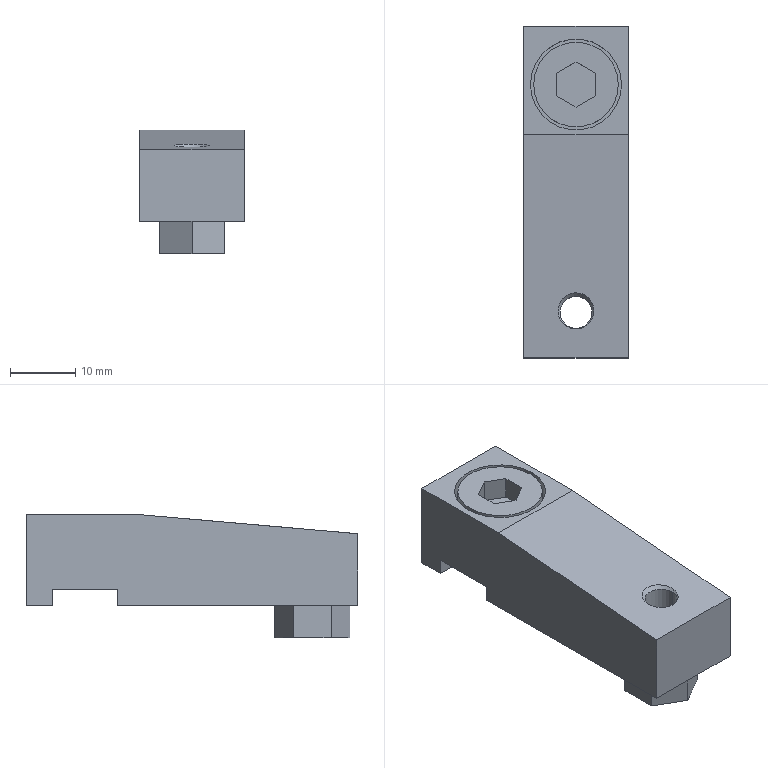Part | SolidWorks | features RefAxis 6, ICE 4, 3DProfileFeature 2, Extrusion 1, RevCut 1, Revolution 1 | 1 solid | 37 faces | box 16 x 51 x 19 mm | volume 10054 mm3 | plane 27 | cylinder 6 | cone 4 | commonest cylinder face diameters 4.917 x2 13 x2 14 x2
STEP:
#1=CARTESIAN_POINT('',(6.5,0.,4.5));
#2=VERTEX_POINT('',#1);
#3=CARTESIAN_POINT('',(-6.5,0.,4.5));
#4=VERTEX_POINT('',#3);
#5=CARTESIAN_POINT('',(0.,0.,4.5));
#6=DIRECTION('',(0.,0.,1.));
#7=DIRECTION('',(1.,0.,0.));
#8=AXIS2_PLACEMENT_3D('',#5,#6,#7);
#9=CIRCLE('',#8,6.5);
#10=EDGE_CURVE('',#2,#4,#9,.T.);
#11=ORIENTED_EDGE('',*,*,#10,.T.);
#12=CARTESIAN_POINT('',(-6.5,0.,11.5));
#13=VERTEX_POINT('',#12);
#14=CARTESIAN_POINT('',(-6.5,0.,4.5));
#15=DIRECTION('',(0.,0.,1.));
#16=VECTOR('',#15,1000.);
#17=LINE('',#14,#16);
#18=EDGE_CURVE('',#4,#13,#17,.T.);
#19=ORIENTED_EDGE('',*,*,#18,.T.);
#20=CARTESIAN_POINT('',(6.5,0.,11.5));
#21=VERTEX_POINT('',#20);
#22=CARTESIAN_POINT('',(0.,0.,11.5));
#23=DIRECTION('',(0.,0.,1.));
#24=DIRECTION('',(1.,0.,0.));
#25=AXIS2_PLACEMENT_3D('',#22,#23,#24);
#26=CIRCLE('',#25,6.5);
#27=EDGE_CURVE('',#21,#13,#26,.T.);
#28=ORIENTED_EDGE('',*,*,#27,.F.);
#29=CARTESIAN_POINT('',(6.5,0.,4.5));
#30=DIRECTION('',(0.,0.,1.));
#31=VECTOR('',#30,1000.);
#32=LINE('',#29,#31);
#33=EDGE_CURVE('',#2,#21,#32,.T.);
#34=ORIENTED_EDGE('',*,*,#33,.F.);
#35=EDGE_LOOP('',(#11,#19,#28,#34));
#36=FACE_OUTER_BOUND('',#35,.T.);
#37=CARTESIAN_POINT('',(0.,0.,4.5));
#38=DIRECTION('',(0.,0.,1.));
#39=DIRECTION('',(1.,0.,0.));
#40=AXIS2_PLACEMENT_3D('',#37,#38,#39);
#41=CYLINDRICAL_SURFACE('',#40,6.5);
#42=ADVANCED_FACE('',(#36),#41,.T.);
#43=CARTESIAN_POINT('',(-7.,0.,4.5));
#44=VERTEX_POINT('',#43);
#45=CARTESIAN_POINT('',(7.,0.,4.5));
#46=VERTEX_POINT('',#45);
#47=CARTESIAN_POINT('',(0.,0.,4.5));
#48=DIRECTION('',(0.,0.,1.));
#49=DIRECTION('',(1.,0.,0.));
#50=AXIS2_PLACEMENT_3D('',#47,#48,#49);
#51=CIRCLE('',#50,7.);
#52=EDGE_CURVE('',#44,#46,#51,.T.);
#53=ORIENTED_EDGE('',*,*,#52,.F.);
#54=CARTESIAN_POINT('',(-7.,0.,11.5));
#55=VERTEX_POINT('',#54);
#56=CARTESIAN_POINT('',(-7.,0.,4.5));
#57=DIRECTION('',(0.,0.,1.));
#58=VECTOR('',#57,1000.);
#59=LINE('',#56,#58);
#60=EDGE_CURVE('',#44,#55,#59,.T.);
#61=ORIENTED_EDGE('',*,*,#60,.T.);
#62=CARTESIAN_POINT('',(7.,0.,11.5));
#63=VERTEX_POINT('',#62);
#64=CARTESIAN_POINT('',(0.,0.,11.5));
#65=DIRECTION('',(0.,0.,1.));
#66=DIRECTION('',(1.,0.,0.));
#67=AXIS2_PLACEMENT_3D('',#64,#65,#66);
#68=CIRCLE('',#67,7.);
#69=EDGE_CURVE('',#55,#63,#68,.T.);
#70=ORIENTED_EDGE('',*,*,#69,.T.);
#71=CARTESIAN_POINT('',(7.,0.,4.5));
#72=DIRECTION('',(0.,0.,1.));
#73=VECTOR('',#72,1000.);
#74=LINE('',#71,#73);
#75=EDGE_CURVE('',#46,#63,#74,.T.);
#76=ORIENTED_EDGE('',*,*,#75,.F.);
#77=EDGE_LOOP('',(#53,#61,#70,#76));
#78=FACE_OUTER_BOUND('',#77,.T.);
#79=CARTESIAN_POINT('',(0.,0.,4.5));
#80=DIRECTION('',(0.,0.,1.));
#81=DIRECTION('',(1.,0.,0.));
#82=AXIS2_PLACEMENT_3D('',#79,#80,#81);
#83=CYLINDRICAL_SURFACE('',#82,7.);
#84=ADVANCED_FACE('',(#78),#83,.F.);
#85=CARTESIAN_POINT('',(-2.459,-35.,-6.959));
#86=VERTEX_POINT('',#85);
#87=CARTESIAN_POINT('',(2.459,-35.,-6.959));
#88=VERTEX_POINT('',#87);
#89=CARTESIAN_POINT('',(0.,-35.,-6.959));
#90=DIRECTION('',(0.,0.,1.));
#91=DIRECTION('',(1.,0.,0.));
#92=AXIS2_PLACEMENT_3D('',#89,#90,#91);
#93=CIRCLE('',#92,2.459);
#94=EDGE_CURVE('',#86,#88,#93,.T.);
#95=ORIENTED_EDGE('',*,*,#94,.F.);
#96=CARTESIAN_POINT('',(-2.459,-35.,8.786));
#97=VERTEX_POINT('',#96);
#98=CARTESIAN_POINT('',(-2.459,-35.,-7.5));
#99=DIRECTION('',(0.,0.,1.));
#100=VECTOR('',#99,1000.);
#101=LINE('',#98,#100);
#102=EDGE_CURVE('',#86,#97,#101,.T.);
#103=ORIENTED_EDGE('',*,*,#102,.T.);
#104=CARTESIAN_POINT('',(2.459,-35.,8.786));
#105=VERTEX_POINT('',#104);
#106=CARTESIAN_POINT('',(0.,-35.,8.786));
#107=DIRECTION('',(0.,0.,1.));
#108=DIRECTION('',(1.,0.,0.));
#109=AXIS2_PLACEMENT_3D('',#106,#107,#108);
#110=CIRCLE('',#109,2.459);
#111=EDGE_CURVE('',#97,#105,#110,.T.);
#112=ORIENTED_EDGE('',*,*,#111,.T.);
#113=CARTESIAN_POINT('',(2.459,-35.,-7.5));
#114=DIRECTION('',(0.,0.,1.));
#115=VECTOR('',#114,1000.);
#116=LINE('',#113,#115);
#117=EDGE_CURVE('',#88,#105,#116,.T.);
#118=ORIENTED_EDGE('',*,*,#117,.F.);
#119=EDGE_LOOP('',(#95,#103,#112,#118));
#120=FACE_OUTER_BOUND('',#119,.T.);
#121=CARTESIAN_POINT('',(0.,-35.,-7.5));
#122=DIRECTION('',(0.,0.,1.));
#123=DIRECTION('',(1.,0.,0.));
#124=AXIS2_PLACEMENT_3D('',#121,#122,#123);
#125=CYLINDRICAL_SURFACE('',#124,2.459);
#126=ADVANCED_FACE('',(#120),#125,.F.);
#127=ORIENTED_EDGE('',*,*,#94,.T.);
#128=CARTESIAN_POINT('',(3.,-35.,-7.5));
#129=VERTEX_POINT('',#128);
#130=CARTESIAN_POINT('',(3.,-35.,-7.5));
#131=DIRECTION('',(0.7071,0.,-0.7071));
#132=VECTOR('',#131,1000.);
#133=LINE('',#130,#132);
#134=EDGE_CURVE('',#88,#129,#133,.T.);
#135=ORIENTED_EDGE('',*,*,#134,.T.);
#136=CARTESIAN_POINT('',(-3.,-35.,-7.5));
#137=VERTEX_POINT('',#136);
#138=CARTESIAN_POINT('',(0.,-35.,-7.5));
#139=DIRECTION('',(0.,0.,1.));
#140=DIRECTION('',(1.,0.,0.));
#141=AXIS2_PLACEMENT_3D('',#138,#139,#140);
#142=CIRCLE('',#141,3.);
#143=EDGE_CURVE('',#137,#129,#142,.T.);
#144=ORIENTED_EDGE('',*,*,#143,.F.);
#145=CARTESIAN_POINT('',(-3.,-35.,-7.5));
#146=DIRECTION('',(-0.7071,0.,-0.7071));
#147=VECTOR('',#146,1000.);
#148=LINE('',#145,#147);
#149=EDGE_CURVE('',#86,#137,#148,.T.);
#150=ORIENTED_EDGE('',*,*,#149,.F.);
#151=EDGE_LOOP('',(#127,#135,#144,#150));
#152=FACE_OUTER_BOUND('',#151,.T.);
#153=CARTESIAN_POINT('',(0.,-35.,-7.5));
#154=DIRECTION('',(0.,0.,-1.));
#155=DIRECTION('',(-1.,0.,0.));
#156=AXIS2_PLACEMENT_3D('',#153,#154,#155);
#157=CONICAL_SURFACE('',#156,3.,0.7854);
#158=ADVANCED_FACE('',(#152),#157,.F.);
#159=ORIENTED_EDGE('',*,*,#111,.F.);
#160=CARTESIAN_POINT('',(-2.759,-35.,9.112));
#161=VERTEX_POINT('',#160);
#162=CARTESIAN_POINT('',(-2.459,-35.,8.786));
#163=DIRECTION('',(-0.6769,0.,0.7361));
#164=VECTOR('',#163,1000.);
#165=LINE('',#162,#164);
#166=EDGE_CURVE('',#97,#161,#165,.T.);
#167=ORIENTED_EDGE('',*,*,#166,.T.);
#168=CARTESIAN_POINT('',(2.759,-35.,9.112));
#169=VERTEX_POINT('',#168);
#170=CARTESIAN_POINT('',(-2.759,-35.,9.112));
#171=CARTESIAN_POINT('',(-2.376,-39.753,8.697));
#172=CARTESIAN_POINT('',(2.376,-39.753,8.697));
#173=CARTESIAN_POINT('',(2.759,-35.,9.112));
#174=(BOUNDED_CURVE()B_SPLINE_CURVE(3,(#170,#171,#172,#173),.UNSPECIFIED.,.F.,.T.)B_SPLINE_CURVE_WITH_KNOTS((4,4),(1.651,4.632),.UNSPECIFIED.)CURVE()GEOMETRIC_REPRESENTATION_ITEM()RATIONAL_B_SPLINE_CURVE((1.,0.387,0.387,1.))REPRESENTATION_ITEM(''));
#175=EDGE_CURVE('',#161,#169,#174,.T.);
#176=ORIENTED_EDGE('',*,*,#175,.T.);
#177=CARTESIAN_POINT('',(2.459,-35.,8.786));
#178=DIRECTION('',(0.6769,0.,0.7361));
#179=VECTOR('',#178,1000.);
#180=LINE('',#177,#179);
#181=EDGE_CURVE('',#105,#169,#180,.T.);
#182=ORIENTED_EDGE('',*,*,#181,.F.);
#183=EDGE_LOOP('',(#159,#167,#176,#182));
#184=FACE_OUTER_BOUND('',#183,.T.);
#185=CARTESIAN_POINT('',(0.,-35.,8.786));
#186=DIRECTION('',(0.,0.,1.));
#187=DIRECTION('',(1.,0.,0.));
#188=AXIS2_PLACEMENT_3D('',#185,#186,#187);
#189=CONICAL_SURFACE('',#188,2.459,0.7435);
#190=ADVANCED_FACE('',(#184),#189,.F.);
#191=CARTESIAN_POINT('',(8.,-7.7,11.5));
#192=VERTEX_POINT('',#191);
#193=CARTESIAN_POINT('',(-8.,-7.7,11.5));
#194=VERTEX_POINT('',#193);
#195=CARTESIAN_POINT('',(8.,-7.7,11.5));
#196=DIRECTION('',(-1.,0.,0.));
#197=VECTOR('',#196,1000.);
#198=LINE('',#195,#197);
#199=EDGE_CURVE('',#192,#194,#198,.T.);
#200=ORIENTED_EDGE('',*,*,#199,.T.);
#201=CARTESIAN_POINT('',(-8.,-42.,8.5));
#202=VERTEX_POINT('',#201);
#203=CARTESIAN_POINT('',(-8.,-7.7,11.5));
#204=DIRECTION('',(0.,-0.9962,-0.08713));
#205=VECTOR('',#204,1000.);
#206=LINE('',#203,#205);
#207=EDGE_CURVE('',#194,#202,#206,.T.);
#208=ORIENTED_EDGE('',*,*,#207,.T.);
#209=CARTESIAN_POINT('',(8.,-42.,8.5));
#210=VERTEX_POINT('',#209);
#211=CARTESIAN_POINT('',(8.,-42.,8.5));
#212=DIRECTION('',(-1.,0.,0.));
#213=VECTOR('',#212,1000.);
#214=LINE('',#211,#213);
#215=EDGE_CURVE('',#210,#202,#214,.T.);
#216=ORIENTED_EDGE('',*,*,#215,.F.);
#217=CARTESIAN_POINT('',(8.,-7.7,11.5));
#218=DIRECTION('',(0.,-0.9962,-0.08713));
#219=VECTOR('',#218,1000.);
#220=LINE('',#217,#219);
#221=EDGE_CURVE('',#192,#210,#220,.T.);
#222=ORIENTED_EDGE('',*,*,#221,.F.);
#223=EDGE_LOOP('',(#200,#208,#216,#222));
#224=FACE_OUTER_BOUND('',#223,.T.);
#225=CARTESIAN_POINT('',(2.759,-35.,9.112));
#226=CARTESIAN_POINT('',(2.898,-33.273,9.263));
#227=CARTESIAN_POINT('',(1.727,-32.,9.375));
#228=CARTESIAN_POINT('',(0.,-32.,9.375));
#229=CARTESIAN_POINT('',(-1.727,-32.,9.375));
#230=CARTESIAN_POINT('',(-2.898,-33.273,9.263));
#231=CARTESIAN_POINT('',(-2.759,-35.,9.112));
#232=(BOUNDED_CURVE()B_SPLINE_CURVE(3,(#225,#226,#227,#228,#229,#230,#231),.UNSPECIFIED.,.F.,.T.)B_SPLINE_CURVE_WITH_KNOTS((4,3,4),(4.632,6.283,7.934),.UNSPECIFIED.)CURVE()GEOMETRIC_REPRESENTATION_ITEM()RATIONAL_B_SPLINE_CURVE((1.,0.7854,0.7854,1.,0.7854,0.7854,1.))REPRESENTATION_ITEM(''));
#233=EDGE_CURVE('',#169,#161,#232,.T.);
#234=ORIENTED_EDGE('',*,*,#233,.F.);
#235=ORIENTED_EDGE('',*,*,#175,.F.);
#236=EDGE_LOOP('',(#234,#235));
#237=FACE_BOUND('',#236,.T.);
#238=CARTESIAN_POINT('',(8.,-7.7,11.5));
#239=DIRECTION('',(0.,0.08713,-0.9962));
#240=DIRECTION('',(0.,0.9962,0.08713));
#241=AXIS2_PLACEMENT_3D('',#238,#239,#240);
#242=PLANE('',#241);
#243=ADVANCED_FACE('',(#224,#237),#242,.F.);
#244=CARTESIAN_POINT('',(4.98,-37.875,-7.5));
#245=VERTEX_POINT('',#244);
#246=CARTESIAN_POINT('',(0.,-40.75,-7.5));
#247=VERTEX_POINT('',#246);
#248=CARTESIAN_POINT('',(4.98,-37.875,-7.5));
#249=DIRECTION('',(-0.866,-0.5,0.));
#250=VECTOR('',#249,1000.);
#251=LINE('',#248,#250);
#252=EDGE_CURVE('',#245,#247,#251,.T.);
#253=ORIENTED_EDGE('',*,*,#252,.T.);
#254=CARTESIAN_POINT('',(-4.98,-37.875,-7.5));
#255=VERTEX_POINT('',#254);
#256=CARTESIAN_POINT('',(0.,-40.75,-7.5));
#257=DIRECTION('',(-0.866,0.5,0.));
#258=VECTOR('',#257,1000.);
#259=LINE('',#256,#258);
#260=EDGE_CURVE('',#247,#255,#259,.T.);
#261=ORIENTED_EDGE('',*,*,#260,.T.);
#262=CARTESIAN_POINT('',(-4.98,-32.125,-7.5));
#263=VERTEX_POINT('',#262);
#264=CARTESIAN_POINT('',(-4.98,-37.875,-7.5));
#265=DIRECTION('',(0.,1.,0.));
#266=VECTOR('',#265,1000.);
#267=LINE('',#264,#266);
#268=EDGE_CURVE('',#255,#263,#267,.T.);
#269=ORIENTED_EDGE('',*,*,#268,.T.);
#270=CARTESIAN_POINT('',(0.,-29.25,-7.5));
#271=VERTEX_POINT('',#270);
#272=CARTESIAN_POINT('',(-4.98,-32.125,-7.5));
#273=DIRECTION('',(0.866,0.5,0.));
#274=VECTOR('',#273,1000.);
#275=LINE('',#272,#274);
#276=EDGE_CURVE('',#263,#271,#275,.T.);
#277=ORIENTED_EDGE('',*,*,#276,.T.);
#278=CARTESIAN_POINT('',(4.98,-32.125,-7.5));
#279=VERTEX_POINT('',#278);
#280=CARTESIAN_POINT('',(0.,-29.25,-7.5));
#281=DIRECTION('',(0.866,-0.5,0.));
#282=VECTOR('',#281,1000.);
#283=LINE('',#280,#282);
#284=EDGE_CURVE('',#271,#279,#283,.T.);
#285=ORIENTED_EDGE('',*,*,#284,.T.);
#286=CARTESIAN_POINT('',(4.98,-32.125,-7.5));
#287=DIRECTION('',(0.,-1.,0.));
#288=VECTOR('',#287,1000.);
#289=LINE('',#286,#288);
#290=EDGE_CURVE('',#279,#245,#289,.T.);
#291=ORIENTED_EDGE('',*,*,#290,.T.);
#292=EDGE_LOOP('',(#253,#261,#269,#277,#285,#291));
#293=FACE_OUTER_BOUND('',#292,.T.);
#294=ORIENTED_EDGE('',*,*,#143,.T.);
#295=CARTESIAN_POINT('',(0.,-35.,-7.5));
#296=DIRECTION('',(0.,0.,1.));
#297=DIRECTION('',(1.,0.,0.));
#298=AXIS2_PLACEMENT_3D('',#295,#296,#297);
#299=CIRCLE('',#298,3.);
#300=EDGE_CURVE('',#129,#137,#299,.T.);
#301=ORIENTED_EDGE('',*,*,#300,.T.);
#302=EDGE_LOOP('',(#294,#301));
#303=FACE_BOUND('',#302,.T.);
#304=CARTESIAN_POINT('',(0.,-29.25,-7.5));
#305=DIRECTION('',(0.,0.,1.));
#306=DIRECTION('',(1.,0.,0.));
#307=AXIS2_PLACEMENT_3D('',#304,#305,#306);
#308=PLANE('',#307);
#309=ADVANCED_FACE('',(#293,#303),#308,.F.);
#310=CARTESIAN_POINT('',(-8.,-5.,-2.5));
#311=VERTEX_POINT('',#310);
#312=CARTESIAN_POINT('',(8.,-5.,-2.5));
#313=VERTEX_POINT('',#312);
#314=CARTESIAN_POINT('',(-8.,-5.,-2.5));
#315=DIRECTION('',(1.,0.,0.));
#316=VECTOR('',#315,1000.);
#317=LINE('',#314,#316);
#318=EDGE_CURVE('',#311,#313,#317,.T.);
#319=ORIENTED_EDGE('',*,*,#318,.T.);
#320=CARTESIAN_POINT('',(8.,-42.,-2.5));
#321=VERTEX_POINT('',#320);
#322=CARTESIAN_POINT('',(8.,-42.,-2.5));
#323=DIRECTION('',(0.,1.,0.));
#324=VECTOR('',#323,1000.);
#325=LINE('',#322,#324);
#326=EDGE_CURVE('',#321,#313,#325,.T.);
#327=ORIENTED_EDGE('',*,*,#326,.F.);
#328=CARTESIAN_POINT('',(-8.,-42.,-2.5));
#329=VERTEX_POINT('',#328);
#330=CARTESIAN_POINT('',(8.,-42.,-2.5));
#331=DIRECTION('',(-1.,0.,0.));
#332=VECTOR('',#331,1000.);
#333=LINE('',#330,#332);
#334=EDGE_CURVE('',#321,#329,#333,.T.);
#335=ORIENTED_EDGE('',*,*,#334,.T.);
#336=CARTESIAN_POINT('',(-8.,-42.,-2.5));
#337=DIRECTION('',(0.,1.,0.));
#338=VECTOR('',#337,1000.);
#339=LINE('',#336,#338);
#340=EDGE_CURVE('',#329,#311,#339,.T.);
#341=ORIENTED_EDGE('',*,*,#340,.T.);
#342=EDGE_LOOP('',(#319,#327,#335,#341));
#343=FACE_OUTER_BOUND('',#342,.T.);
#344=CARTESIAN_POINT('',(0.,-40.75,-2.5));
#345=VERTEX_POINT('',#344);
#346=CARTESIAN_POINT('',(-4.98,-37.875,-2.5));
#347=VERTEX_POINT('',#346);
#348=CARTESIAN_POINT('',(0.,-40.75,-2.5));
#349=DIRECTION('',(-0.866,0.5,0.));
#350=VECTOR('',#349,1000.);
#351=LINE('',#348,#350);
#352=EDGE_CURVE('',#345,#347,#351,.T.);
#353=ORIENTED_EDGE('',*,*,#352,.F.);
#354=CARTESIAN_POINT('',(4.98,-37.875,-2.5));
#355=VERTEX_POINT('',#354);
#356=CARTESIAN_POINT('',(4.98,-37.875,-2.5));
#357=DIRECTION('',(-0.866,-0.5,0.));
#358=VECTOR('',#357,1000.);
#359=LINE('',#356,#358);
#360=EDGE_CURVE('',#355,#345,#359,.T.);
#361=ORIENTED_EDGE('',*,*,#360,.F.);
#362=CARTESIAN_POINT('',(4.98,-32.125,-2.5));
#363=VERTEX_POINT('',#362);
#364=CARTESIAN_POINT('',(4.98,-32.125,-2.5));
#365=DIRECTION('',(0.,-1.,0.));
#366=VECTOR('',#365,1000.);
#367=LINE('',#364,#366);
#368=EDGE_CURVE('',#363,#355,#367,.T.);
#369=ORIENTED_EDGE('',*,*,#368,.F.);
#370=CARTESIAN_POINT('',(0.,-29.25,-2.5));
#371=VERTEX_POINT('',#370);
#372=CARTESIAN_POINT('',(0.,-29.25,-2.5));
#373=DIRECTION('',(0.866,-0.5,0.));
#374=VECTOR('',#373,1000.);
#375=LINE('',#372,#374);
#376=EDGE_CURVE('',#371,#363,#375,.T.);
#377=ORIENTED_EDGE('',*,*,#376,.F.);
#378=CARTESIAN_POINT('',(-4.98,-32.125,-2.5));
#379=VERTEX_POINT('',#378);
#380=CARTESIAN_POINT('',(-4.98,-32.125,-2.5));
#381=DIRECTION('',(0.866,0.5,0.));
#382=VECTOR('',#381,1000.);
#383=LINE('',#380,#382);
#384=EDGE_CURVE('',#379,#371,#383,.T.);
#385=ORIENTED_EDGE('',*,*,#384,.F.);
#386=CARTESIAN_POINT('',(-4.98,-37.875,-2.5));
#387=DIRECTION('',(0.,1.,0.));
#388=VECTOR('',#387,1000.);
#389=LINE('',#386,#388);
#390=EDGE_CURVE('',#347,#379,#389,.T.);
#391=ORIENTED_EDGE('',*,*,#390,.F.);
#392=EDGE_LOOP('',(#353,#361,#369,#377,#385,#391));
#393=FACE_BOUND('',#392,.T.);
#394=CARTESIAN_POINT('',(8.,-42.,-2.5));
#395=DIRECTION('',(0.,0.,1.));
#396=DIRECTION('',(1.,0.,0.));
#397=AXIS2_PLACEMENT_3D('',#394,#395,#396);
#398=PLANE('',#397);
#399=ADVANCED_FACE('',(#343,#393),#398,.F.);
#400=CARTESIAN_POINT('',(8.,5.,-2.5));
#401=VERTEX_POINT('',#400);
#402=CARTESIAN_POINT('',(8.,9.,-2.5));
#403=VERTEX_POINT('',#402);
#404=CARTESIAN_POINT('',(8.,-42.,-2.5));
#405=DIRECTION('',(0.,1.,0.));
#406=VECTOR('',#405,1000.);
#407=LINE('',#404,#406);
#408=EDGE_CURVE('',#401,#403,#407,.T.);
#409=ORIENTED_EDGE('',*,*,#408,.F.);
#410=CARTESIAN_POINT('',(-8.,5.,-2.5));
#411=VERTEX_POINT('',#410);
#412=CARTESIAN_POINT('',(8.,5.,-2.5));
#413=DIRECTION('',(-1.,0.,0.));
#414=VECTOR('',#413,1000.);
#415=LINE('',#412,#414);
#416=EDGE_CURVE('',#401,#411,#415,.T.);
#417=ORIENTED_EDGE('',*,*,#416,.T.);
#418=CARTESIAN_POINT('',(-8.,9.,-2.5));
#419=VERTEX_POINT('',#418);
#420=CARTESIAN_POINT('',(-8.,-42.,-2.5));
#421=DIRECTION('',(0.,1.,0.));
#422=VECTOR('',#421,1000.);
#423=LINE('',#420,#422);
#424=EDGE_CURVE('',#411,#419,#423,.T.);
#425=ORIENTED_EDGE('',*,*,#424,.T.);
#426=CARTESIAN_POINT('',(8.,9.,-2.5));
#427=DIRECTION('',(-1.,0.,0.));
#428=VECTOR('',#427,1000.);
#429=LINE('',#426,#428);
#430=EDGE_CURVE('',#403,#419,#429,.T.);
#431=ORIENTED_EDGE('',*,*,#430,.F.);
#432=EDGE_LOOP('',(#409,#417,#425,#431));
#433=FACE_OUTER_BOUND('',#432,.T.);
#434=CARTESIAN_POINT('',(8.,-42.,-2.5));
#435=DIRECTION('',(0.,0.,1.));
#436=DIRECTION('',(1.,0.,0.));
#437=AXIS2_PLACEMENT_3D('',#434,#435,#436);
#438=PLANE('',#437);
#439=ADVANCED_FACE('',(#433),#438,.F.);
#440=ORIENTED_EDGE('',*,*,#430,.T.);
#441=CARTESIAN_POINT('',(-8.,9.,11.5));
#442=VERTEX_POINT('',#441);
#443=CARTESIAN_POINT('',(-8.,9.,-2.5));
#444=DIRECTION('',(0.,0.,1.));
#445=VECTOR('',#444,1000.);
#446=LINE('',#443,#445);
#447=EDGE_CURVE('',#419,#442,#446,.T.);
#448=ORIENTED_EDGE('',*,*,#447,.T.);
#449=CARTESIAN_POINT('',(8.,9.,11.5));
#450=VERTEX_POINT('',#449);
#451=CARTESIAN_POINT('',(8.,9.,11.5));
#452=DIRECTION('',(-1.,0.,0.));
#453=VECTOR('',#452,1000.);
#454=LINE('',#451,#453);
#455=EDGE_CURVE('',#450,#442,#454,.T.);
#456=ORIENTED_EDGE('',*,*,#455,.F.);
#457=CARTESIAN_POINT('',(8.,9.,-2.5));
#458=DIRECTION('',(0.,0.,1.));
#459=VECTOR('',#458,1000.);
#460=LINE('',#457,#459);
#461=EDGE_CURVE('',#403,#450,#460,.T.);
#462=ORIENTED_EDGE('',*,*,#461,.F.);
#463=EDGE_LOOP('',(#440,#448,#456,#462));
#464=FACE_OUTER_BOUND('',#463,.T.);
#465=CARTESIAN_POINT('',(8.,9.,-2.5));
#466=DIRECTION('',(0.,-1.,0.));
#467=DIRECTION('',(0.,0.,-1.));
#468=AXIS2_PLACEMENT_3D('',#465,#466,#467);
#469=PLANE('',#468);
#470=ADVANCED_FACE('',(#464),#469,.F.);
#471=CARTESIAN_POINT('',(0.,0.,11.5));
#472=DIRECTION('',(0.,0.,1.));
#473=DIRECTION('',(1.,0.,0.));
#474=AXIS2_PLACEMENT_3D('',#471,#472,#473);
#475=CIRCLE('',#474,7.);
#476=EDGE_CURVE('',#63,#55,#475,.T.);
#477=ORIENTED_EDGE('',*,*,#476,.F.);
#478=ORIENTED_EDGE('',*,*,#69,.F.);
#479=EDGE_LOOP('',(#477,#478));
#480=FACE_BOUND('',#479,.T.);
#481=ORIENTED_EDGE('',*,*,#455,.T.);
#482=CARTESIAN_POINT('',(-8.,9.,11.5));
#483=DIRECTION('',(0.,-1.,0.));
#484=VECTOR('',#483,1000.);
#485=LINE('',#482,#484);
#486=EDGE_CURVE('',#442,#194,#485,.T.);
#487=ORIENTED_EDGE('',*,*,#486,.T.);
#488=ORIENTED_EDGE('',*,*,#199,.F.);
#489=CARTESIAN_POINT('',(8.,9.,11.5));
#490=DIRECTION('',(0.,-1.,0.));
#491=VECTOR('',#490,1000.);
#492=LINE('',#489,#491);
#493=EDGE_CURVE('',#450,#192,#492,.T.);
#494=ORIENTED_EDGE('',*,*,#493,.F.);
#495=EDGE_LOOP('',(#481,#487,#488,#494));
#496=FACE_OUTER_BOUND('',#495,.T.);
#497=CARTESIAN_POINT('',(8.,9.,11.5));
#498=DIRECTION('',(0.,0.,-1.));
#499=DIRECTION('',(-1.,0.,0.));
#500=AXIS2_PLACEMENT_3D('',#497,#498,#499);
#501=PLANE('',#500);
#502=ADVANCED_FACE('',(#480,#496),#501,.F.);
#503=ORIENTED_EDGE('',*,*,#215,.T.);
#504=CARTESIAN_POINT('',(-8.,-42.,8.5));
#505=DIRECTION('',(0.,0.,-1.));
#506=VECTOR('',#505,1000.);
#507=LINE('',#504,#506);
#508=EDGE_CURVE('',#202,#329,#507,.T.);
#509=ORIENTED_EDGE('',*,*,#508,.T.);
#510=ORIENTED_EDGE('',*,*,#334,.F.);
#511=CARTESIAN_POINT('',(8.,-42.,8.5));
#512=DIRECTION('',(0.,0.,-1.));
#513=VECTOR('',#512,1000.);
#514=LINE('',#511,#513);
#515=EDGE_CURVE('',#210,#321,#514,.T.);
#516=ORIENTED_EDGE('',*,*,#515,.F.);
#517=EDGE_LOOP('',(#503,#509,#510,#516));
#518=FACE_OUTER_BOUND('',#517,.T.);
#519=CARTESIAN_POINT('',(8.,-42.,8.5));
#520=DIRECTION('',(0.,1.,0.));
#521=DIRECTION('',(0.,0.,1.));
#522=AXIS2_PLACEMENT_3D('',#519,#520,#521);
#523=PLANE('',#522);
#524=ADVANCED_FACE('',(#518),#523,.F.);
#525=CARTESIAN_POINT('',(8.,5.,0.));
#526=VERTEX_POINT('',#525);
#527=CARTESIAN_POINT('',(8.,5.,-2.5));
#528=DIRECTION('',(0.,0.,1.));
#529=VECTOR('',#528,1000.);
#530=LINE('',#527,#529);
#531=EDGE_CURVE('',#401,#526,#530,.T.);
#532=ORIENTED_EDGE('',*,*,#531,.F.);
#533=ORIENTED_EDGE('',*,*,#408,.T.);
#534=ORIENTED_EDGE('',*,*,#461,.T.);
#535=ORIENTED_EDGE('',*,*,#493,.T.);
#536=ORIENTED_EDGE('',*,*,#221,.T.);
#537=ORIENTED_EDGE('',*,*,#515,.T.);
#538=ORIENTED_EDGE('',*,*,#326,.T.);
#539=CARTESIAN_POINT('',(8.,-5.,0.));
#540=VERTEX_POINT('',#539);
#541=CARTESIAN_POINT('',(8.,-5.,-2.5));
#542=DIRECTION('',(0.,0.,1.));
#543=VECTOR('',#542,1000.);
#544=LINE('',#541,#543);
#545=EDGE_CURVE('',#313,#540,#544,.T.);
#546=ORIENTED_EDGE('',*,*,#545,.T.);
#547=CARTESIAN_POINT('',(8.,-5.,0.));
#548=DIRECTION('',(0.,1.,0.));
#549=VECTOR('',#548,1000.);
#550=LINE('',#547,#549);
#551=EDGE_CURVE('',#540,#526,#550,.T.);
#552=ORIENTED_EDGE('',*,*,#551,.T.);
#553=EDGE_LOOP('',(#532,#533,#534,#535,#536,#537,#538,#546,#552));
#554=FACE_OUTER_BOUND('',#553,.T.);
#555=CARTESIAN_POINT('',(8.,0.,0.));
#556=DIRECTION('',(1.,0.,0.));
#557=DIRECTION('',(0.,0.,-1.));
#558=AXIS2_PLACEMENT_3D('',#555,#556,#557);
#559=PLANE('',#558);
#560=ADVANCED_FACE('',(#554),#559,.T.);
#561=ORIENTED_EDGE('',*,*,#424,.F.);
#562=CARTESIAN_POINT('',(-8.,5.,0.));
#563=VERTEX_POINT('',#562);
#564=CARTESIAN_POINT('',(-8.,5.,-2.5));
#565=DIRECTION('',(0.,0.,1.));
#566=VECTOR('',#565,1000.);
#567=LINE('',#564,#566);
#568=EDGE_CURVE('',#411,#563,#567,.T.);
#569=ORIENTED_EDGE('',*,*,#568,.T.);
#570=CARTESIAN_POINT('',(-8.,-5.,0.));
#571=VERTEX_POINT('',#570);
#572=CARTESIAN_POINT('',(-8.,5.,0.));
#573=DIRECTION('',(0.,-1.,0.));
#574=VECTOR('',#573,1000.);
#575=LINE('',#572,#574);
#576=EDGE_CURVE('',#563,#571,#575,.T.);
#577=ORIENTED_EDGE('',*,*,#576,.T.);
#578=CARTESIAN_POINT('',(-8.,-5.,-2.5));
#579=DIRECTION('',(0.,0.,1.));
#580=VECTOR('',#579,1000.);
#581=LINE('',#578,#580);
#582=EDGE_CURVE('',#311,#571,#581,.T.);
#583=ORIENTED_EDGE('',*,*,#582,.F.);
#584=ORIENTED_EDGE('',*,*,#340,.F.);
#585=ORIENTED_EDGE('',*,*,#508,.F.);
#586=ORIENTED_EDGE('',*,*,#207,.F.);
#587=ORIENTED_EDGE('',*,*,#486,.F.);
#588=ORIENTED_EDGE('',*,*,#447,.F.);
#589=EDGE_LOOP('',(#561,#569,#577,#583,#584,#585,#586,#587,#588));
#590=FACE_OUTER_BOUND('',#589,.T.);
#591=CARTESIAN_POINT('',(-8.,0.,0.));
#592=DIRECTION('',(1.,0.,0.));
#593=DIRECTION('',(0.,0.,-1.));
#594=AXIS2_PLACEMENT_3D('',#591,#592,#593);
#595=PLANE('',#594);
#596=ADVANCED_FACE('',(#590),#595,.F.);
#597=CARTESIAN_POINT('',(8.,5.,0.));
#598=DIRECTION('',(-1.,0.,0.));
#599=VECTOR('',#598,1000.);
#600=LINE('',#597,#599);
#601=EDGE_CURVE('',#526,#563,#600,.T.);
#602=ORIENTED_EDGE('',*,*,#601,.T.);
#603=ORIENTED_EDGE('',*,*,#568,.F.);
#604=ORIENTED_EDGE('',*,*,#416,.F.);
#605=ORIENTED_EDGE('',*,*,#531,.T.);
#606=EDGE_LOOP('',(#602,#603,#604,#605));
#607=FACE_OUTER_BOUND('',#606,.T.);
#608=CARTESIAN_POINT('',(8.,5.,-2.5));
#609=DIRECTION('',(0.,1.,0.));
#610=DIRECTION('',(0.,0.,1.));
#611=AXIS2_PLACEMENT_3D('',#608,#609,#610);
#612=PLANE('',#611);
#613=ADVANCED_FACE('',(#607),#612,.F.);
#614=CARTESIAN_POINT('',(-8.,-5.,0.));
#615=DIRECTION('',(1.,0.,0.));
#616=VECTOR('',#615,1000.);
#617=LINE('',#614,#616);
#618=EDGE_CURVE('',#571,#540,#617,.T.);
#619=ORIENTED_EDGE('',*,*,#618,.T.);
#620=ORIENTED_EDGE('',*,*,#545,.F.);
#621=ORIENTED_EDGE('',*,*,#318,.F.);
#622=ORIENTED_EDGE('',*,*,#582,.T.);
#623=EDGE_LOOP('',(#619,#620,#621,#622));
#624=FACE_OUTER_BOUND('',#623,.T.);
#625=CARTESIAN_POINT('',(-8.,-5.,-2.5));
#626=DIRECTION('',(0.,-1.,0.));
#627=DIRECTION('',(0.,0.,-1.));
#628=AXIS2_PLACEMENT_3D('',#625,#626,#627);
#629=PLANE('',#628);
#630=ADVANCED_FACE('',(#624),#629,.F.);
#631=ORIENTED_EDGE('',*,*,#601,.F.);
#632=ORIENTED_EDGE('',*,*,#551,.F.);
#633=ORIENTED_EDGE('',*,*,#618,.F.);
#634=ORIENTED_EDGE('',*,*,#576,.F.);
#635=EDGE_LOOP('',(#631,#632,#633,#634));
#636=FACE_OUTER_BOUND('',#635,.T.);
#637=CARTESIAN_POINT('',(0.,0.,0.));
#638=DIRECTION('',(0.,0.,1.));
#639=DIRECTION('',(1.,0.,0.));
#640=AXIS2_PLACEMENT_3D('',#637,#638,#639);
#641=PLANE('',#640);
#642=ADVANCED_FACE('',(#636),#641,.F.);
#643=ORIENTED_EDGE('',*,*,#252,.F.);
#644=CARTESIAN_POINT('',(4.98,-37.875,-2.5));
#645=DIRECTION('',(0.,0.,-1.));
#646=VECTOR('',#645,1000.);
#647=LINE('',#644,#646);
#648=EDGE_CURVE('',#355,#245,#647,.T.);
#649=ORIENTED_EDGE('',*,*,#648,.F.);
#650=ORIENTED_EDGE('',*,*,#360,.T.);
#651=CARTESIAN_POINT('',(0.,-40.75,-2.5));
#652=DIRECTION('',(0.,0.,-1.));
#653=VECTOR('',#652,1000.);
#654=LINE('',#651,#653);
#655=EDGE_CURVE('',#345,#247,#654,.T.);
#656=ORIENTED_EDGE('',*,*,#655,.T.);
#657=EDGE_LOOP('',(#643,#649,#650,#656));
#658=FACE_OUTER_BOUND('',#657,.T.);
#659=CARTESIAN_POINT('',(4.98,-37.875,-2.5));
#660=DIRECTION('',(0.5,-0.866,0.));
#661=DIRECTION('',(0.866,0.5,0.));
#662=AXIS2_PLACEMENT_3D('',#659,#660,#661);
#663=PLANE('',#662);
#664=ADVANCED_FACE('',(#658),#663,.T.);
#665=ORIENTED_EDGE('',*,*,#290,.F.);
#666=CARTESIAN_POINT('',(4.98,-32.125,-2.5));
#667=DIRECTION('',(0.,0.,-1.));
#668=VECTOR('',#667,1000.);
#669=LINE('',#666,#668);
#670=EDGE_CURVE('',#363,#279,#669,.T.);
#671=ORIENTED_EDGE('',*,*,#670,.F.);
#672=ORIENTED_EDGE('',*,*,#368,.T.);
#673=ORIENTED_EDGE('',*,*,#648,.T.);
#674=EDGE_LOOP('',(#665,#671,#672,#673));
#675=FACE_OUTER_BOUND('',#674,.T.);
#676=CARTESIAN_POINT('',(4.98,-32.125,-2.5));
#677=DIRECTION('',(1.,0.,0.));
#678=DIRECTION('',(0.,0.,-1.));
#679=AXIS2_PLACEMENT_3D('',#676,#677,#678);
#680=PLANE('',#679);
#681=ADVANCED_FACE('',(#675),#680,.T.);
#682=ORIENTED_EDGE('',*,*,#284,.F.);
#683=CARTESIAN_POINT('',(0.,-29.25,-2.5));
#684=DIRECTION('',(0.,0.,-1.));
#685=VECTOR('',#684,1000.);
#686=LINE('',#683,#685);
#687=EDGE_CURVE('',#371,#271,#686,.T.);
#688=ORIENTED_EDGE('',*,*,#687,.F.);
#689=ORIENTED_EDGE('',*,*,#376,.T.);
#690=ORIENTED_EDGE('',*,*,#670,.T.);
#691=EDGE_LOOP('',(#682,#688,#689,#690));
#692=FACE_OUTER_BOUND('',#691,.T.);
#693=CARTESIAN_POINT('',(0.,-29.25,-2.5));
#694=DIRECTION('',(0.5,0.866,0.));
#695=DIRECTION('',(-0.866,0.5,0.));
#696=AXIS2_PLACEMENT_3D('',#693,#694,#695);
#697=PLANE('',#696);
#698=ADVANCED_FACE('',(#692),#697,.T.);
#699=ORIENTED_EDGE('',*,*,#276,.F.);
#700=CARTESIAN_POINT('',(-4.98,-32.125,-2.5));
#701=DIRECTION('',(0.,0.,-1.));
#702=VECTOR('',#701,1000.);
#703=LINE('',#700,#702);
#704=EDGE_CURVE('',#379,#263,#703,.T.);
#705=ORIENTED_EDGE('',*,*,#704,.F.);
#706=ORIENTED_EDGE('',*,*,#384,.T.);
#707=ORIENTED_EDGE('',*,*,#687,.T.);
#708=EDGE_LOOP('',(#699,#705,#706,#707));
#709=FACE_OUTER_BOUND('',#708,.T.);
#710=CARTESIAN_POINT('',(-4.98,-32.125,-2.5));
#711=DIRECTION('',(-0.5,0.866,0.));
#712=DIRECTION('',(-0.866,-0.5,0.));
#713=AXIS2_PLACEMENT_3D('',#710,#711,#712);
#714=PLANE('',#713);
#715=ADVANCED_FACE('',(#709),#714,.T.);
#716=ORIENTED_EDGE('',*,*,#268,.F.);
#717=CARTESIAN_POINT('',(-4.98,-37.875,-2.5));
#718=DIRECTION('',(0.,0.,-1.));
#719=VECTOR('',#718,1000.);
#720=LINE('',#717,#719);
#721=EDGE_CURVE('',#347,#255,#720,.T.);
#722=ORIENTED_EDGE('',*,*,#721,.F.);
#723=ORIENTED_EDGE('',*,*,#390,.T.);
#724=ORIENTED_EDGE('',*,*,#704,.T.);
#725=EDGE_LOOP('',(#716,#722,#723,#724));
#726=FACE_OUTER_BOUND('',#725,.T.);
#727=CARTESIAN_POINT('',(-4.98,-37.875,-2.5));
#728=DIRECTION('',(-1.,0.,0.));
#729=DIRECTION('',(0.,0.,1.));
#730=AXIS2_PLACEMENT_3D('',#727,#728,#729);
#731=PLANE('',#730);
#732=ADVANCED_FACE('',(#726),#731,.T.);
#733=ORIENTED_EDGE('',*,*,#260,.F.);
#734=ORIENTED_EDGE('',*,*,#655,.F.);
#735=ORIENTED_EDGE('',*,*,#352,.T.);
#736=ORIENTED_EDGE('',*,*,#721,.T.);
#737=EDGE_LOOP('',(#733,#734,#735,#736));
#738=FACE_OUTER_BOUND('',#737,.T.);
#739=CARTESIAN_POINT('',(0.,-40.75,-2.5));
#740=DIRECTION('',(-0.5,-0.866,0.));
#741=DIRECTION('',(0.866,-0.5,0.));
#742=AXIS2_PLACEMENT_3D('',#739,#740,#741);
#743=PLANE('',#742);
#744=ADVANCED_FACE('',(#738),#743,.T.);
#745=ORIENTED_EDGE('',*,*,#166,.F.);
#746=CARTESIAN_POINT('',(0.,-35.,8.786));
#747=DIRECTION('',(0.,0.,1.));
#748=DIRECTION('',(1.,0.,0.));
#749=AXIS2_PLACEMENT_3D('',#746,#747,#748);
#750=CIRCLE('',#749,2.459);
#751=EDGE_CURVE('',#105,#97,#750,.T.);
#752=ORIENTED_EDGE('',*,*,#751,.F.);
#753=ORIENTED_EDGE('',*,*,#181,.T.);
#754=ORIENTED_EDGE('',*,*,#233,.T.);
#755=EDGE_LOOP('',(#745,#752,#753,#754));
#756=FACE_OUTER_BOUND('',#755,.T.);
#757=CARTESIAN_POINT('',(0.,-35.,8.786));
#758=DIRECTION('',(0.,0.,1.));
#759=DIRECTION('',(1.,0.,0.));
#760=AXIS2_PLACEMENT_3D('',#757,#758,#759);
#761=CONICAL_SURFACE('',#760,2.459,0.7435);
#762=ADVANCED_FACE('',(#756),#761,.F.);
#763=ORIENTED_EDGE('',*,*,#134,.F.);
#764=CARTESIAN_POINT('',(0.,-35.,-6.959));
#765=DIRECTION('',(0.,0.,1.));
#766=DIRECTION('',(1.,0.,0.));
#767=AXIS2_PLACEMENT_3D('',#764,#765,#766);
#768=CIRCLE('',#767,2.459);
#769=EDGE_CURVE('',#88,#86,#768,.T.);
#770=ORIENTED_EDGE('',*,*,#769,.T.);
#771=ORIENTED_EDGE('',*,*,#149,.T.);
#772=ORIENTED_EDGE('',*,*,#300,.F.);
#773=EDGE_LOOP('',(#763,#770,#771,#772));
#774=FACE_OUTER_BOUND('',#773,.T.);
#775=CARTESIAN_POINT('',(0.,-35.,-7.5));
#776=DIRECTION('',(0.,0.,-1.));
#777=DIRECTION('',(-1.,0.,0.));
#778=AXIS2_PLACEMENT_3D('',#775,#776,#777);
#779=CONICAL_SURFACE('',#778,3.,0.7854);
#780=ADVANCED_FACE('',(#774),#779,.F.);
#781=ORIENTED_EDGE('',*,*,#102,.F.);
#782=ORIENTED_EDGE('',*,*,#769,.F.);
#783=ORIENTED_EDGE('',*,*,#117,.T.);
#784=ORIENTED_EDGE('',*,*,#751,.T.);
#785=EDGE_LOOP('',(#781,#782,#783,#784));
#786=FACE_OUTER_BOUND('',#785,.T.);
#787=CARTESIAN_POINT('',(0.,-35.,-7.5));
#788=DIRECTION('',(0.,0.,1.));
#789=DIRECTION('',(1.,0.,0.));
#790=AXIS2_PLACEMENT_3D('',#787,#788,#789);
#791=CYLINDRICAL_SURFACE('',#790,2.459);
#792=ADVANCED_FACE('',(#786),#791,.F.);
#793=ORIENTED_EDGE('',*,*,#60,.F.);
#794=CARTESIAN_POINT('',(0.,0.,4.5));
#795=DIRECTION('',(0.,0.,1.));
#796=DIRECTION('',(1.,0.,0.));
#797=AXIS2_PLACEMENT_3D('',#794,#795,#796);
#798=CIRCLE('',#797,7.);
#799=EDGE_CURVE('',#46,#44,#798,.T.);
#800=ORIENTED_EDGE('',*,*,#799,.F.);
#801=ORIENTED_EDGE('',*,*,#75,.T.);
#802=ORIENTED_EDGE('',*,*,#476,.T.);
#803=EDGE_LOOP('',(#793,#800,#801,#802));
#804=FACE_OUTER_BOUND('',#803,.T.);
#805=CARTESIAN_POINT('',(0.,0.,4.5));
#806=DIRECTION('',(0.,0.,1.));
#807=DIRECTION('',(1.,0.,0.));
#808=AXIS2_PLACEMENT_3D('',#805,#806,#807);
#809=CYLINDRICAL_SURFACE('',#808,7.);
#810=ADVANCED_FACE('',(#804),#809,.F.);
#811=ORIENTED_EDGE('',*,*,#10,.F.);
#812=CARTESIAN_POINT('',(0.,0.,4.5));
#813=DIRECTION('',(0.,0.,1.));
#814=DIRECTION('',(1.,0.,0.));
#815=AXIS2_PLACEMENT_3D('',#812,#813,#814);
#816=CIRCLE('',#815,6.5);
#817=EDGE_CURVE('',#4,#2,#816,.T.);
#818=ORIENTED_EDGE('',*,*,#817,.F.);
#819=EDGE_LOOP('',(#811,#818));
#820=FACE_BOUND('',#819,.T.);
#821=ORIENTED_EDGE('',*,*,#799,.T.);
#822=ORIENTED_EDGE('',*,*,#52,.T.);
#823=EDGE_LOOP('',(#821,#822));
#824=FACE_OUTER_BOUND('',#823,.T.);
#825=CARTESIAN_POINT('',(0.,0.,4.5));
#826=DIRECTION('',(0.,0.,1.));
#827=DIRECTION('',(1.,0.,0.));
#828=AXIS2_PLACEMENT_3D('',#825,#826,#827);
#829=PLANE('',#828);
#830=ADVANCED_FACE('',(#820,#824),#829,.T.);
#831=ORIENTED_EDGE('',*,*,#18,.F.);
#832=ORIENTED_EDGE('',*,*,#817,.T.);
#833=ORIENTED_EDGE('',*,*,#33,.T.);
#834=CARTESIAN_POINT('',(0.,0.,11.5));
#835=DIRECTION('',(0.,0.,1.));
#836=DIRECTION('',(1.,0.,0.));
#837=AXIS2_PLACEMENT_3D('',#834,#835,#836);
#838=CIRCLE('',#837,6.5);
#839=EDGE_CURVE('',#13,#21,#838,.T.);
#840=ORIENTED_EDGE('',*,*,#839,.F.);
#841=EDGE_LOOP('',(#831,#832,#833,#840));
#842=FACE_OUTER_BOUND('',#841,.T.);
#843=CARTESIAN_POINT('',(0.,0.,4.5));
#844=DIRECTION('',(0.,0.,1.));
#845=DIRECTION('',(1.,0.,0.));
#846=AXIS2_PLACEMENT_3D('',#843,#844,#845);
#847=CYLINDRICAL_SURFACE('',#846,6.5);
#848=ADVANCED_FACE('',(#842),#847,.T.);
#849=CARTESIAN_POINT('',(-3.,1.732,11.5));
#850=VERTEX_POINT('',#849);
#851=CARTESIAN_POINT('',(-3.,-1.732,11.5));
#852=VERTEX_POINT('',#851);
#853=CARTESIAN_POINT('',(-3.,1.732,11.5));
#854=DIRECTION('',(0.,-1.,0.));
#855=VECTOR('',#854,1000.);
#856=LINE('',#853,#855);
#857=EDGE_CURVE('',#850,#852,#856,.T.);
#858=ORIENTED_EDGE('',*,*,#857,.F.);
#859=CARTESIAN_POINT('',(0.,3.464,11.5));
#860=VERTEX_POINT('',#859);
#861=CARTESIAN_POINT('',(0.,3.464,11.5));
#862=DIRECTION('',(-0.866,-0.5,0.));
#863=VECTOR('',#862,1000.);
#864=LINE('',#861,#863);
#865=EDGE_CURVE('',#860,#850,#864,.T.);
#866=ORIENTED_EDGE('',*,*,#865,.F.);
#867=CARTESIAN_POINT('',(3.,1.732,11.5));
#868=VERTEX_POINT('',#867);
#869=CARTESIAN_POINT('',(3.,1.732,11.5));
#870=DIRECTION('',(-0.866,0.5,0.));
#871=VECTOR('',#870,1000.);
#872=LINE('',#869,#871);
#873=EDGE_CURVE('',#868,#860,#872,.T.);
#874=ORIENTED_EDGE('',*,*,#873,.F.);
#875=CARTESIAN_POINT('',(3.,-1.732,11.5));
#876=VERTEX_POINT('',#875);
#877=CARTESIAN_POINT('',(3.,-1.732,11.5));
#878=DIRECTION('',(0.,1.,0.));
#879=VECTOR('',#878,1000.);
#880=LINE('',#877,#879);
#881=EDGE_CURVE('',#876,#868,#880,.T.);
#882=ORIENTED_EDGE('',*,*,#881,.F.);
#883=CARTESIAN_POINT('',(0.,-3.464,11.5));
#884=VERTEX_POINT('',#883);
#885=CARTESIAN_POINT('',(0.,-3.464,11.5));
#886=DIRECTION('',(0.866,0.5,0.));
#887=VECTOR('',#886,1000.);
#888=LINE('',#885,#887);
#889=EDGE_CURVE('',#884,#876,#888,.T.);
#890=ORIENTED_EDGE('',*,*,#889,.F.);
#891=CARTESIAN_POINT('',(-3.,-1.732,11.5));
#892=DIRECTION('',(0.866,-0.5,0.));
#893=VECTOR('',#892,1000.);
#894=LINE('',#891,#893);
#895=EDGE_CURVE('',#852,#884,#894,.T.);
#896=ORIENTED_EDGE('',*,*,#895,.F.);
#897=EDGE_LOOP('',(#858,#866,#874,#882,#890,#896));
#898=FACE_BOUND('',#897,.T.);
#899=ORIENTED_EDGE('',*,*,#27,.T.);
#900=ORIENTED_EDGE('',*,*,#839,.T.);
#901=EDGE_LOOP('',(#899,#900));
#902=FACE_OUTER_BOUND('',#901,.T.);
#903=CARTESIAN_POINT('',(8.,9.,11.5));
#904=DIRECTION('',(0.,0.,-1.));
#905=DIRECTION('',(-1.,0.,0.));
#906=AXIS2_PLACEMENT_3D('',#903,#904,#905);
#907=PLANE('',#906);
#908=ADVANCED_FACE('',(#898,#902),#907,.F.);
#909=ORIENTED_EDGE('',*,*,#865,.T.);
#910=CARTESIAN_POINT('',(-3.,1.732,8.));
#911=VERTEX_POINT('',#910);
#912=CARTESIAN_POINT('',(-3.,1.732,8.));
#913=DIRECTION('',(0.,0.,1.));
#914=VECTOR('',#913,1000.);
#915=LINE('',#912,#914);
#916=EDGE_CURVE('',#911,#850,#915,.T.);
#917=ORIENTED_EDGE('',*,*,#916,.F.);
#918=CARTESIAN_POINT('',(0.,3.464,8.));
#919=VERTEX_POINT('',#918);
#920=CARTESIAN_POINT('',(0.,3.464,8.));
#921=DIRECTION('',(-0.866,-0.5,0.));
#922=VECTOR('',#921,1000.);
#923=LINE('',#920,#922);
#924=EDGE_CURVE('',#919,#911,#923,.T.);
#925=ORIENTED_EDGE('',*,*,#924,.F.);
#926=CARTESIAN_POINT('',(0.,3.464,8.));
#927=DIRECTION('',(0.,0.,1.));
#928=VECTOR('',#927,1000.);
#929=LINE('',#926,#928);
#930=EDGE_CURVE('',#919,#860,#929,.T.);
#931=ORIENTED_EDGE('',*,*,#930,.T.);
#932=EDGE_LOOP('',(#909,#917,#925,#931));
#933=FACE_OUTER_BOUND('',#932,.T.);
#934=CARTESIAN_POINT('',(0.,3.464,8.));
#935=DIRECTION('',(-0.5,0.866,0.));
#936=DIRECTION('',(-0.866,-0.5,0.));
#937=AXIS2_PLACEMENT_3D('',#934,#935,#936);
#938=PLANE('',#937);
#939=ADVANCED_FACE('',(#933),#938,.F.);
#940=ORIENTED_EDGE('',*,*,#873,.T.);
#941=ORIENTED_EDGE('',*,*,#930,.F.);
#942=CARTESIAN_POINT('',(3.,1.732,8.));
#943=VERTEX_POINT('',#942);
#944=CARTESIAN_POINT('',(3.,1.732,8.));
#945=DIRECTION('',(-0.866,0.5,0.));
#946=VECTOR('',#945,1000.);
#947=LINE('',#944,#946);
#948=EDGE_CURVE('',#943,#919,#947,.T.);
#949=ORIENTED_EDGE('',*,*,#948,.F.);
#950=CARTESIAN_POINT('',(3.,1.732,8.));
#951=DIRECTION('',(0.,0.,1.));
#952=VECTOR('',#951,1000.);
#953=LINE('',#950,#952);
#954=EDGE_CURVE('',#943,#868,#953,.T.);
#955=ORIENTED_EDGE('',*,*,#954,.T.);
#956=EDGE_LOOP('',(#940,#941,#949,#955));
#957=FACE_OUTER_BOUND('',#956,.T.);
#958=CARTESIAN_POINT('',(3.,1.732,8.));
#959=DIRECTION('',(0.5,0.866,0.));
#960=DIRECTION('',(-0.866,0.5,0.));
#961=AXIS2_PLACEMENT_3D('',#958,#959,#960);
#962=PLANE('',#961);
#963=ADVANCED_FACE('',(#957),#962,.F.);
#964=ORIENTED_EDGE('',*,*,#881,.T.);
#965=ORIENTED_EDGE('',*,*,#954,.F.);
#966=CARTESIAN_POINT('',(3.,-1.732,8.));
#967=VERTEX_POINT('',#966);
#968=CARTESIAN_POINT('',(3.,-1.732,8.));
#969=DIRECTION('',(0.,1.,0.));
#970=VECTOR('',#969,1000.);
#971=LINE('',#968,#970);
#972=EDGE_CURVE('',#967,#943,#971,.T.);
#973=ORIENTED_EDGE('',*,*,#972,.F.);
#974=CARTESIAN_POINT('',(3.,-1.732,8.));
#975=DIRECTION('',(0.,0.,1.));
#976=VECTOR('',#975,1000.);
#977=LINE('',#974,#976);
#978=EDGE_CURVE('',#967,#876,#977,.T.);
#979=ORIENTED_EDGE('',*,*,#978,.T.);
#980=EDGE_LOOP('',(#964,#965,#973,#979));
#981=FACE_OUTER_BOUND('',#980,.T.);
#982=CARTESIAN_POINT('',(3.,-1.732,8.));
#983=DIRECTION('',(1.,0.,0.));
#984=DIRECTION('',(0.,0.,-1.));
#985=AXIS2_PLACEMENT_3D('',#982,#983,#984);
#986=PLANE('',#985);
#987=ADVANCED_FACE('',(#981),#986,.F.);
#988=ORIENTED_EDGE('',*,*,#889,.T.);
#989=ORIENTED_EDGE('',*,*,#978,.F.);
#990=CARTESIAN_POINT('',(0.,-3.464,8.));
#991=VERTEX_POINT('',#990);
#992=CARTESIAN_POINT('',(0.,-3.464,8.));
#993=DIRECTION('',(0.866,0.5,0.));
#994=VECTOR('',#993,1000.);
#995=LINE('',#992,#994);
#996=EDGE_CURVE('',#991,#967,#995,.T.);
#997=ORIENTED_EDGE('',*,*,#996,.F.);
#998=CARTESIAN_POINT('',(0.,-3.464,8.));
#999=DIRECTION('',(0.,0.,1.));
#1000=VECTOR('',#999,1000.);
#1001=LINE('',#998,#1000);
#1002=EDGE_CURVE('',#991,#884,#1001,.T.);
#1003=ORIENTED_EDGE('',*,*,#1002,.T.);
#1004=EDGE_LOOP('',(#988,#989,#997,#1003));
#1005=FACE_OUTER_BOUND('',#1004,.T.);
#1006=CARTESIAN_POINT('',(0.,-3.464,8.));
#1007=DIRECTION('',(0.5,-0.866,0.));
#1008=DIRECTION('',(0.866,0.5,0.));
#1009=AXIS2_PLACEMENT_3D('',#1006,#1007,#1008);
#1010=PLANE('',#1009);
#1011=ADVANCED_FACE('',(#1005),#1010,.F.);
#1012=ORIENTED_EDGE('',*,*,#895,.T.);
#1013=ORIENTED_EDGE('',*,*,#1002,.F.);
#1014=CARTESIAN_POINT('',(-3.,-1.732,8.));
#1015=VERTEX_POINT('',#1014);
#1016=CARTESIAN_POINT('',(-3.,-1.732,8.));
#1017=DIRECTION('',(0.866,-0.5,0.));
#1018=VECTOR('',#1017,1000.);
#1019=LINE('',#1016,#1018);
#1020=EDGE_CURVE('',#1015,#991,#1019,.T.);
#1021=ORIENTED_EDGE('',*,*,#1020,.F.);
#1022=CARTESIAN_POINT('',(-3.,-1.732,8.));
#1023=DIRECTION('',(0.,0.,1.));
#1024=VECTOR('',#1023,1000.);
#1025=LINE('',#1022,#1024);
#1026=EDGE_CURVE('',#1015,#852,#1025,.T.);
#1027=ORIENTED_EDGE('',*,*,#1026,.T.);
#1028=EDGE_LOOP('',(#1012,#1013,#1021,#1027));
#1029=FACE_OUTER_BOUND('',#1028,.T.);
#1030=CARTESIAN_POINT('',(-3.,-1.732,8.));
#1031=DIRECTION('',(-0.5,-0.866,0.));
#1032=DIRECTION('',(0.866,-0.5,0.));
#1033=AXIS2_PLACEMENT_3D('',#1030,#1031,#1032);
#1034=PLANE('',#1033);
#1035=ADVANCED_FACE('',(#1029),#1034,.F.);
#1036=ORIENTED_EDGE('',*,*,#857,.T.);
#1037=ORIENTED_EDGE('',*,*,#1026,.F.);
#1038=CARTESIAN_POINT('',(-3.,1.732,8.));
#1039=DIRECTION('',(0.,-1.,0.));
#1040=VECTOR('',#1039,1000.);
#1041=LINE('',#1038,#1040);
#1042=EDGE_CURVE('',#911,#1015,#1041,.T.);
#1043=ORIENTED_EDGE('',*,*,#1042,.F.);
#1044=ORIENTED_EDGE('',*,*,#916,.T.);
#1045=EDGE_LOOP('',(#1036,#1037,#1043,#1044));
#1046=FACE_OUTER_BOUND('',#1045,.T.);
#1047=CARTESIAN_POINT('',(-3.,1.732,8.));
#1048=DIRECTION('',(-1.,0.,0.));
#1049=DIRECTION('',(0.,0.,1.));
#1050=AXIS2_PLACEMENT_3D('',#1047,#1048,#1049);
#1051=PLANE('',#1050);
#1052=ADVANCED_FACE('',(#1046),#1051,.F.);
#1053=ORIENTED_EDGE('',*,*,#924,.T.);
#1054=ORIENTED_EDGE('',*,*,#1042,.T.);
#1055=ORIENTED_EDGE('',*,*,#1020,.T.);
#1056=ORIENTED_EDGE('',*,*,#996,.T.);
#1057=ORIENTED_EDGE('',*,*,#972,.T.);
#1058=ORIENTED_EDGE('',*,*,#948,.T.);
#1059=EDGE_LOOP('',(#1053,#1054,#1055,#1056,#1057,#1058));
#1060=FACE_OUTER_BOUND('',#1059,.T.);
#1061=CARTESIAN_POINT('',(0.,0.,8.));
#1062=DIRECTION('',(0.,0.,1.));
#1063=DIRECTION('',(1.,0.,0.));
#1064=AXIS2_PLACEMENT_3D('',#1061,#1062,#1063);
#1065=PLANE('',#1064);
#1066=ADVANCED_FACE('',(#1060),#1065,.T.);
#1067=CLOSED_SHELL('',(#42,#84,#126,#158,#190,#243,#309,#399,#439,#470,#502,#524,#560,#596,#613,#630,#642,#664,#681,#698,#715,#732,#744,#762,#780,#792,#810,#830,#848,#908,#939,#963,#987,#1011,#1035,#1052,#1066));
#1068=MANIFOLD_SOLID_BREP('',#1067);
#1069=CARTESIAN_POINT('',(0.,0.,0.));
#1070=DIRECTION('',(0.,0.,1.));
#1071=DIRECTION('',(1.,0.,0.));
#1072=AXIS2_PLACEMENT_3D('',#1069,#1070,#1071);
#1073=(LENGTH_UNIT()NAMED_UNIT(*)SI_UNIT(.MILLI.,.METRE.));
#1074=UNCERTAINTY_MEASURE_WITH_UNIT(LENGTH_MEASURE(0.00001),#1073,'','');
#1075=(NAMED_UNIT(*)PLANE_ANGLE_UNIT()SI_UNIT($,.RADIAN.));
#1076=(NAMED_UNIT(*)SI_UNIT($,.STERADIAN.)SOLID_ANGLE_UNIT());
#1077=(GEOMETRIC_REPRESENTATION_CONTEXT(3)GLOBAL_UNCERTAINTY_ASSIGNED_CONTEXT((#1074))GLOBAL_UNIT_ASSIGNED_CONTEXT((#1073,#1075,#1076))REPRESENTATION_CONTEXT('',''));
#1078=ADVANCED_BREP_SHAPE_REPRESENTATION('',(#1068,#1072),#1077);